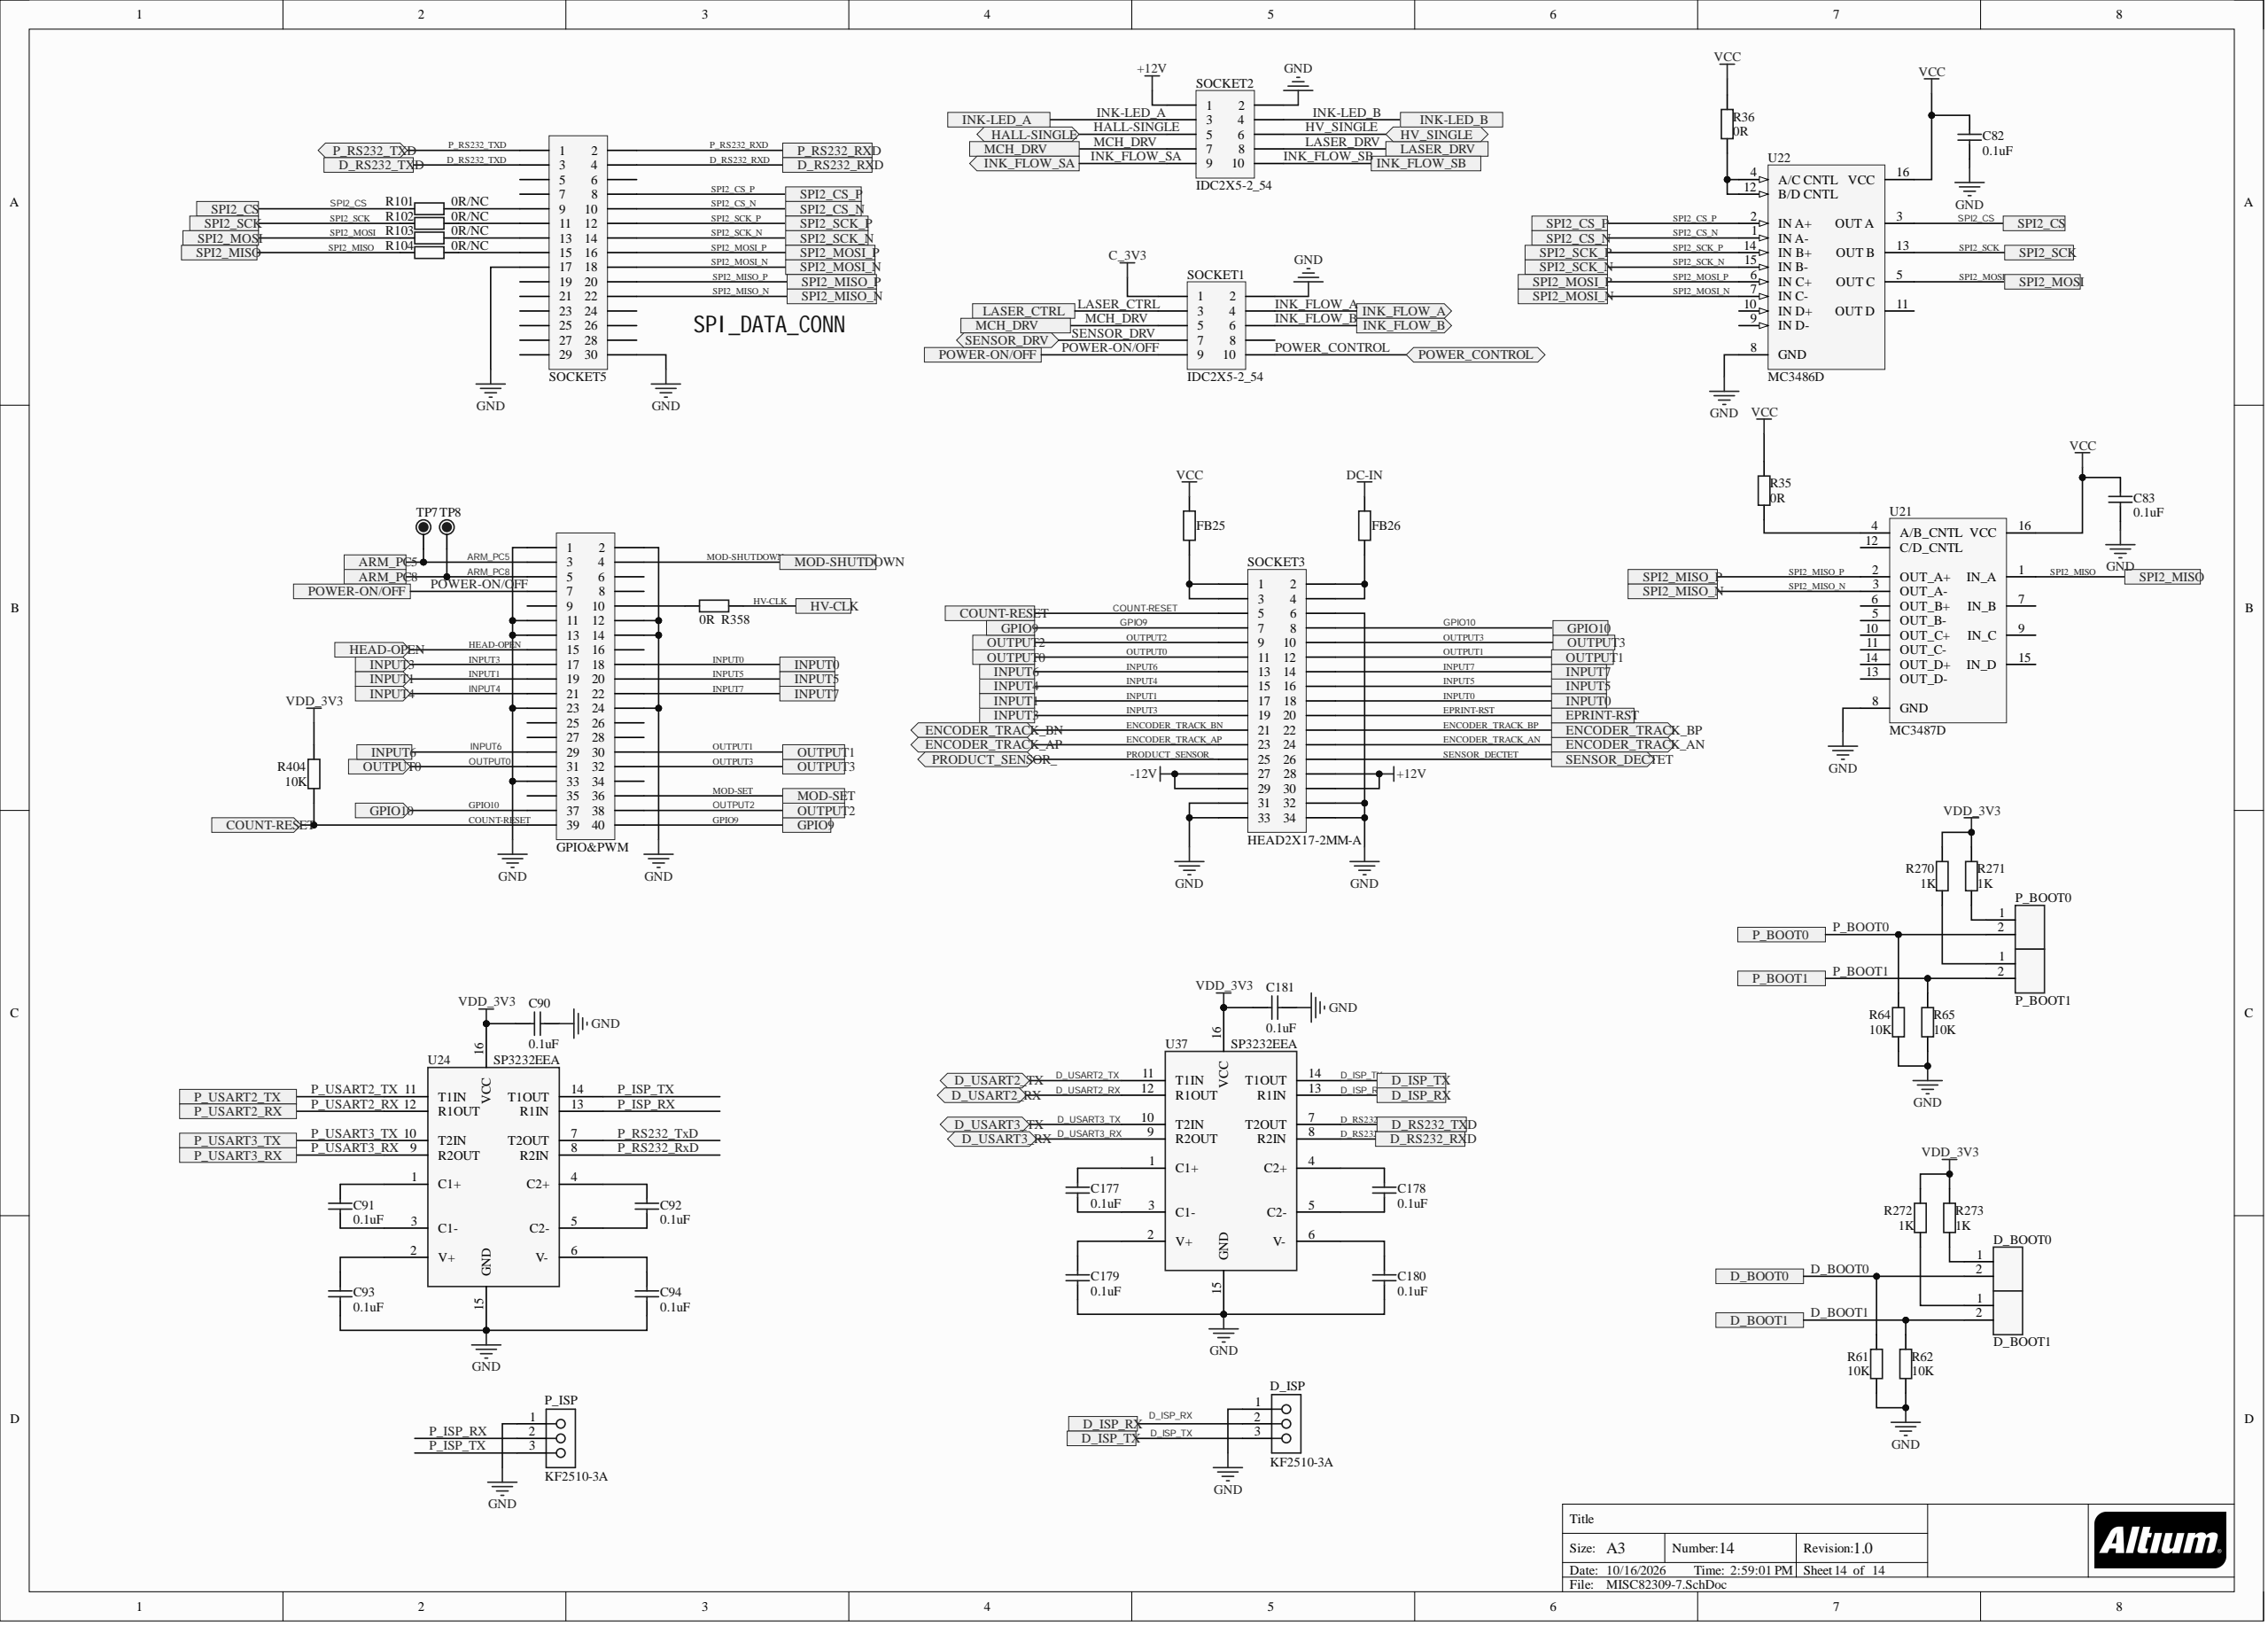Circuit board | Altium Designer | 747 parts | 576 nets | one sheet of the schematic
Parts on this sheet (reference | value | footprint):
C82 | 0.1uF | CAP_0805
C83 | 0.1uF | CAP_0805
C90 | 0.1uF | C0603
C91 | 0.1uF | C0603
C92 | 0.1uF | C0603
C93 | 0.1uF | C0603
C94 | 0.1uF | C0603
C177 | 0.1uF | C0603
C178 | 0.1uF | C0603
C179 | 0.1uF | C0603
C180 | 0.1uF | C0603
C181 | 0.1uF | C0603
D_ISP | KF2510-3A | KF2510-3A
FB25 | 60 | SMD1206-L
FB26 | 60 | SMD1206-L
GPIO&PWM | HEAD2X20-2MM-A | IDC2X20-2.0mm-A
P_ISP | KF2510-3A | KF2510-3A
R35 | 0R | RES_0603
R36 | 0R | RES_0603
R61 | 10K | RES_0603
R62 | 10K | RES_0603
R64 | 10K | RES_0603
R65 | 10K | RES_0603
R101 | 0R/NC | RES_0603
R102 | 0R/NC | RES_0603
R103 | 0R/NC | RES_0603
R104 | 0R/NC | RES_0603
R270 | 1K | RES_0603
R271 | 1K | RES_0603
R272 | 1K | RES_0603
R273 | 1K | RES_0603
R358 | 0R | RES_0603
R404 | 10K | RES_0603
SOCKET1 | IDC2X5-2_54 | IDC2X5-2_54
SOCKET2 | IDC2X5-2_54 | IDC2X5-2_54
SOCKET3 | HEAD2X17-2MM-A | IDC2X17-2.0mm-A
SOCKET5 | HEAD2X15-2MM-A | IDC2X15-2.0mm-A
U21 | MC3487D | 751B-03_N
U22 | MC3486D | 751B-03_N
U24 | SP3232EEA | SSOP16_M
U37 | SP3232EEA | SSOP16_M
Nets of these parts (net: part-pin ...):
VDD_3V3: C90-2 C181-2 R270-2 R271-2 R272-2 R273-2 R404-1 U24-16 U37-16
VCC: C82-2 C83-2 FB25-1 R35-2 R36-2 U21-16 U22-16
SPI2_SCK_P: SOCKET5-12 U22-14
SPI2_SCK_N: SOCKET5-14 U22-15
SPI2_MOSI_P: SOCKET5-16 U22-6
SPI2_MOSI_N: SOCKET5-18 U22-7
SPI2_MOSI: R103-1 U22-5
SPI2_MISO_P: SOCKET5-20 U21-2
SPI2_MISO_N: SOCKET5-22 U21-3
SPI2_CS_P: SOCKET5-8 U22-2
SPI2_CS_N: SOCKET5-10 U22-1
SPI2_CS: R101-1 U22-3
SENSOR_DRV: SOCKET1-7
SENSOR_DECTET: SOCKET3-26
PRODUCT_SENSOR_: SOCKET3-25
POWER_CONTROL: SOCKET1-10
POWER-ON/OFF: SOCKET1-9 GPIO&PWM-7
P_USART3_TX: U24-10
P_USART3_RX: U24-9
P_USART2_TX: U24-11
P_USART2_RX: U24-12
P_RS232_TxD: SOCKET5-1 U24-7
P_RS232_RxD: SOCKET5-2 U24-8
P_JTDO: R102-1 U22-13
P_JNTRST: R104-1 U21-1
P_ISP_TX: P_ISP-3 U24-14
P_ISP_RX: P_ISP-2 U24-13
P_BOOT1: R65-1
P_BOOT0: R64-1
OUTPUT3: GPIO&PWM-32 SOCKET3-10
OUTPUT2: GPIO&PWM-38 SOCKET3-9
OUTPUT1: GPIO&PWM-30 SOCKET3-12
OUTPUT0: GPIO&PWM-31 SOCKET3-11
NetR104_2: R104-2 SOCKET5-15
NetR103_2: R103-2 SOCKET5-13
NetR102_2: R102-2 SOCKET5-11
NetR101_2: R101-2 SOCKET5-9
NetR36_1: R36-1 U22-4 U22-12
NetR35_1: R35-1 U21-4
NetP_BOOT1_1: R270-1
NetP_BOOT0_1: R271-1
NetGPIO&PWM_10: R358-1 GPIO&PWM-10
NetFB26_2: FB26-2 SOCKET3-2 SOCKET3-4
NetFB25_2: FB25-2 SOCKET3-1 SOCKET3-3
NetD_BOOT1_1: R272-1
NetD_BOOT0_1: R273-1
NetC180_2: C180-2 U37-6
NetC179_2: C179-2 U37-2
NetC178_2: C178-2 U37-4
NetC178_1: C178-1 U37-5
NetC177_2: C177-2 U37-1
NetC177_1: C177-1 U37-3
NetC94_2: C94-2 U24-6
NetC93_2: C93-2 U24-2
NetC92_2: C92-2 U24-4
NetC92_1: C92-1 U24-5
NetC91_2: C91-2 U24-1
NetC91_1: C91-1 U24-3
MOD-SHUTDOWN: GPIO&PWM-4
MOD-SET: GPIO&PWM-36
MCH_DRV: SOCKET1-5 SOCKET2-7
LASER_DRV: SOCKET2-8
LASER_CTRL: SOCKET1-3
INPUT7: GPIO&PWM-22 SOCKET3-14
INPUT6: GPIO&PWM-29 SOCKET3-13
INPUT5: GPIO&PWM-20 SOCKET3-16
INPUT4: GPIO&PWM-21 SOCKET3-15
INPUT3: GPIO&PWM-17 SOCKET3-19
INPUT1: GPIO&PWM-19 SOCKET3-17
INPUT0: GPIO&PWM-18 SOCKET3-18
INK_FLOW_SB: SOCKET2-10
INK_FLOW_SA: SOCKET2-9
INK_FLOW_B: SOCKET1-6
INK_FLOW_A: SOCKET1-4
INK-LED_B: SOCKET2-4
INK-LED_A: SOCKET2-3
HV_SINGLE: SOCKET2-6
HV-CLK: R358-2
HEAD-OPEN: GPIO&PWM-15
HALL-SINGLE: SOCKET2-5
GPIO10: GPIO&PWM-37 SOCKET3-8
GPIO9: GPIO&PWM-40 SOCKET3-7
GND: C82-1 C83-1 C90-1 C93-1 C94-1 C179-1 C180-1 C181-1 D_ISP-1 P_ISP-1 R61-2 R62-2 R64-2 R65-2 SOCKET1-2 SOCKET2-2 SOCKET5-17 SOCKET5-30 U21-8 U22-8 U24-15 U37-15 GPIO&PWM-1 GPIO&PWM-2 GPIO&PWM-11 GPIO&PWM-12 GPIO&PWM-13 GPIO&PWM-14 GPIO&PWM-23 GPIO&PWM-24 GPIO&PWM-33 SOCKET3-6 SOCKET3-31 SOCKET3-32 SOCKET3-33 SOCKET3-34
EPRINT-RST: SOCKET3-20
ENCODER_TRACK_BP: SOCKET3-22
ENCODER_TRACK_BN: SOCKET3-21
ENCODER_TRACK_AP: SOCKET3-23
ENCODER_TRACK_AN: SOCKET3-24
DC-IN: FB26-1
D_USART3_TX: U37-10
D_USART3_RX: U37-9
D_USART2_TX: U37-11
D_USART2_RX: U37-12
D_RS232_TXD: SOCKET5-3 U37-7
D_RS232_RXD: SOCKET5-4 U37-8
D_ISP_TX: D_ISP-3 U37-14
D_ISP_RX: D_ISP-2 U37-13
D_BOOT1: R62-1
D_BOOT0: R61-1
COUNT-RESET: R404-2 GPIO&PWM-39 SOCKET3-5
C_3V3: SOCKET1-1
ARM_PC8: GPIO&PWM-5
ARM_PC5: GPIO&PWM-3
-12V: SOCKET3-27 SOCKET3-29
+12V: SOCKET2-1 SOCKET3-28 SOCKET3-30